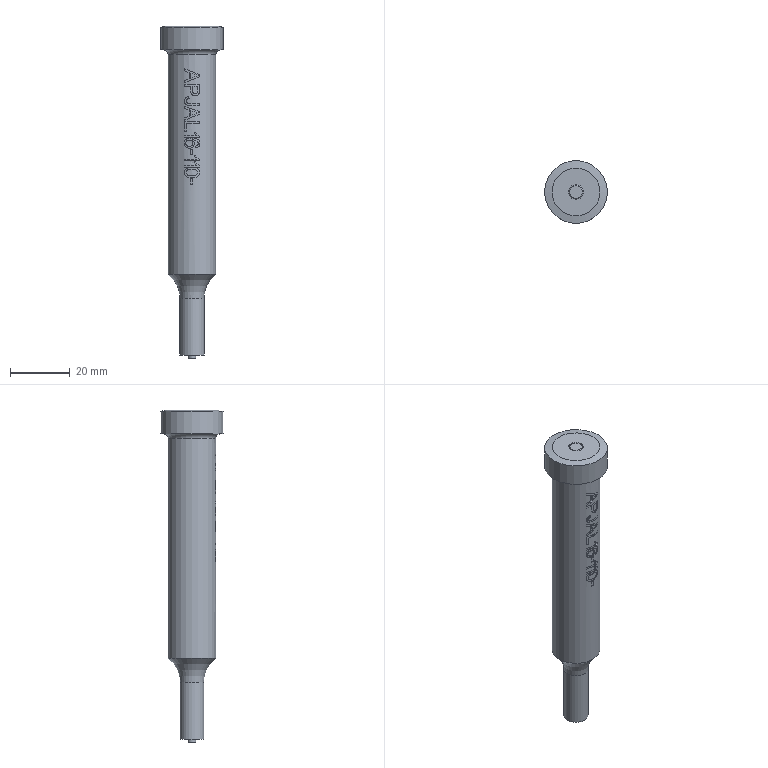Part | NX | features APJAL16-110-P10.00_2 2 | 1 solid | 144 faces | box 21 x 21 x 111 mm | volume 19409 mm3 | plane 87 | cylinder 52 | torus 2 | cone 2 | spline 1 | commonest cylinder face diameters 15.8 x12 16 x6 6.337 x3 7.115 x3 1.507 x1 1.757 x1